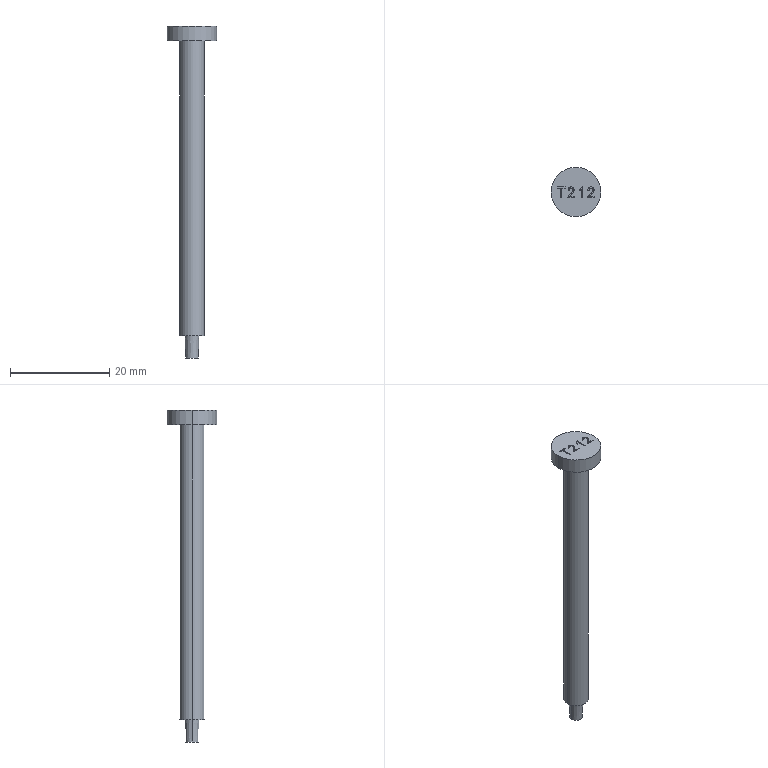Part | Creo | 1 solid | 75 faces | box 10 x 10 x 67.028 mm | volume 1429 mm3 | other 40 | plane 27 | cylinder 6 | cone 2 | commonest cylinder face diameters 1.927 x2 5 x2 10 x2